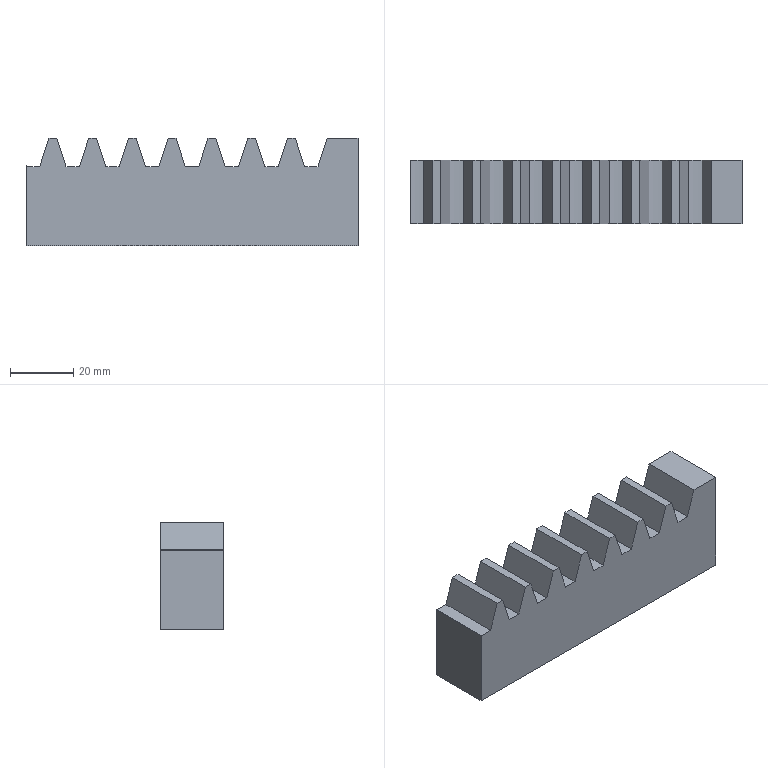Part | SolidWorks | features BaseBody 1 | 1 solid | 37 faces | box 104.88 x 20 x 34 mm | volume 61301 mm3 | plane 29 | cylinder 8 | commonest cylinder face diameters 94.224 x8
STEP:
#1=CARTESIAN_POINT('',(-7.679,369.5,-110.95));
#2=VERTEX_POINT('',#1);
#3=CARTESIAN_POINT('',(-7.753,369.5,-110.721));
#4=VERTEX_POINT('',#3);
#5=CARTESIAN_POINT('',(-7.679,369.5,-110.95));
#6=DIRECTION('',(-0.3083,0.,0.9513));
#7=VECTOR('',#6,1000.);
#8=LINE('',#5,#7);
#9=EDGE_CURVE('',#2,#4,#8,.T.);
#10=ORIENTED_EDGE('',*,*,#9,.T.);
#11=CARTESIAN_POINT('',(-7.753,369.5,-136.));
#12=VERTEX_POINT('',#11);
#13=CARTESIAN_POINT('',(-7.753,369.5,-55.957));
#14=DIRECTION('',(0.,0.,-1.));
#15=VECTOR('',#14,1000.);
#16=LINE('',#13,#15);
#17=EDGE_CURVE('',#4,#12,#16,.T.);
#18=ORIENTED_EDGE('',*,*,#17,.T.);
#19=CARTESIAN_POINT('',(97.127,369.5,-136.));
#20=VERTEX_POINT('',#19);
#21=CARTESIAN_POINT('',(52.127,369.5,-136.));
#22=DIRECTION('',(1.,0.,0.));
#23=VECTOR('',#22,1000.);
#24=LINE('',#21,#23);
#25=EDGE_CURVE('',#12,#20,#24,.T.);
#26=ORIENTED_EDGE('',*,*,#25,.T.);
#27=CARTESIAN_POINT('',(97.127,369.5,-102.));
#28=VERTEX_POINT('',#27);
#29=CARTESIAN_POINT('',(97.127,369.5,-55.957));
#30=DIRECTION('',(0.,0.,1.));
#31=VECTOR('',#30,1000.);
#32=LINE('',#29,#31);
#33=EDGE_CURVE('',#20,#28,#32,.T.);
#34=ORIENTED_EDGE('',*,*,#33,.T.);
#35=CARTESIAN_POINT('',(87.393,369.5,-102.));
#36=VERTEX_POINT('',#35);
#37=CARTESIAN_POINT('',(52.127,369.5,-102.));
#38=DIRECTION('',(-1.,0.,0.));
#39=VECTOR('',#38,1000.);
#40=LINE('',#37,#39);
#41=EDGE_CURVE('',#28,#36,#40,.T.);
#42=ORIENTED_EDGE('',*,*,#41,.T.);
#43=CARTESIAN_POINT('',(84.492,369.5,-110.95));
#44=VERTEX_POINT('',#43);
#45=CARTESIAN_POINT('',(97.545,369.5,-70.676));
#46=DIRECTION('',(-0.3083,0.,-0.9513));
#47=VECTOR('',#46,1000.);
#48=LINE('',#45,#47);
#49=EDGE_CURVE('',#36,#44,#48,.T.);
#50=ORIENTED_EDGE('',*,*,#49,.T.);
#51=CARTESIAN_POINT('',(80.241,369.5,-110.95));
#52=VERTEX_POINT('',#51);
#53=CARTESIAN_POINT('',(82.367,369.5,-63.886));
#54=DIRECTION('',(0.,1.,0.));
#55=DIRECTION('',(0.,0.,1.));
#56=AXIS2_PLACEMENT_3D('',#53,#54,#55);
#57=CIRCLE('',#56,47.112);
#58=EDGE_CURVE('',#44,#52,#57,.T.);
#59=ORIENTED_EDGE('',*,*,#58,.T.);
#60=CARTESIAN_POINT('',(77.34,369.5,-102.));
#61=VERTEX_POINT('',#60);
#62=CARTESIAN_POINT('',(80.241,369.5,-110.95));
#63=DIRECTION('',(-0.3083,0.,0.9513));
#64=VECTOR('',#63,1000.);
#65=LINE('',#62,#64);
#66=EDGE_CURVE('',#52,#61,#65,.T.);
#67=ORIENTED_EDGE('',*,*,#66,.T.);
#68=CARTESIAN_POINT('',(74.833,369.5,-102.));
#69=VERTEX_POINT('',#68);
#70=CARTESIAN_POINT('',(52.127,369.5,-102.));
#71=DIRECTION('',(-1.,0.,0.));
#72=VECTOR('',#71,1000.);
#73=LINE('',#70,#72);
#74=EDGE_CURVE('',#61,#69,#73,.T.);
#75=ORIENTED_EDGE('',*,*,#74,.T.);
#76=CARTESIAN_POINT('',(71.932,369.5,-110.95));
#77=VERTEX_POINT('',#76);
#78=CARTESIAN_POINT('',(86.178,369.5,-66.992));
#79=DIRECTION('',(-0.3083,0.,-0.9513));
#80=VECTOR('',#79,1000.);
#81=LINE('',#78,#80);
#82=EDGE_CURVE('',#69,#77,#81,.T.);
#83=ORIENTED_EDGE('',*,*,#82,.T.);
#84=CARTESIAN_POINT('',(67.681,369.5,-110.95));
#85=VERTEX_POINT('',#84);
#86=CARTESIAN_POINT('',(69.807,369.5,-63.886));
#87=DIRECTION('',(0.,1.,0.));
#88=DIRECTION('',(0.,0.,1.));
#89=AXIS2_PLACEMENT_3D('',#86,#87,#88);
#90=CIRCLE('',#89,47.112);
#91=EDGE_CURVE('',#77,#85,#90,.T.);
#92=ORIENTED_EDGE('',*,*,#91,.T.);
#93=CARTESIAN_POINT('',(64.78,369.5,-102.));
#94=VERTEX_POINT('',#93);
#95=CARTESIAN_POINT('',(67.681,369.5,-110.95));
#96=DIRECTION('',(-0.3083,0.,0.9513));
#97=VECTOR('',#96,1000.);
#98=LINE('',#95,#97);
#99=EDGE_CURVE('',#85,#94,#98,.T.);
#100=ORIENTED_EDGE('',*,*,#99,.T.);
#101=CARTESIAN_POINT('',(62.273,369.5,-102.));
#102=VERTEX_POINT('',#101);
#103=CARTESIAN_POINT('',(52.127,369.5,-102.));
#104=DIRECTION('',(-1.,0.,0.));
#105=VECTOR('',#104,1000.);
#106=LINE('',#103,#105);
#107=EDGE_CURVE('',#94,#102,#106,.T.);
#108=ORIENTED_EDGE('',*,*,#107,.T.);
#109=CARTESIAN_POINT('',(59.372,369.5,-110.95));
#110=VERTEX_POINT('',#109);
#111=CARTESIAN_POINT('',(74.812,369.5,-63.309));
#112=DIRECTION('',(-0.3083,0.,-0.9513));
#113=VECTOR('',#112,1000.);
#114=LINE('',#111,#113);
#115=EDGE_CURVE('',#102,#110,#114,.T.);
#116=ORIENTED_EDGE('',*,*,#115,.T.);
#117=CARTESIAN_POINT('',(55.121,369.5,-110.95));
#118=VERTEX_POINT('',#117);
#119=CARTESIAN_POINT('',(57.247,369.5,-63.886));
#120=DIRECTION('',(0.,1.,0.));
#121=DIRECTION('',(0.,0.,1.));
#122=AXIS2_PLACEMENT_3D('',#119,#120,#121);
#123=CIRCLE('',#122,47.112);
#124=EDGE_CURVE('',#110,#118,#123,.T.);
#125=ORIENTED_EDGE('',*,*,#124,.T.);
#126=CARTESIAN_POINT('',(52.22,369.5,-102.));
#127=VERTEX_POINT('',#126);
#128=CARTESIAN_POINT('',(55.121,369.5,-110.95));
#129=DIRECTION('',(-0.3083,0.,0.9513));
#130=VECTOR('',#129,1000.);
#131=LINE('',#128,#130);
#132=EDGE_CURVE('',#118,#127,#131,.T.);
#133=ORIENTED_EDGE('',*,*,#132,.T.);
#134=CARTESIAN_POINT('',(49.713,369.5,-102.));
#135=VERTEX_POINT('',#134);
#136=CARTESIAN_POINT('',(52.127,369.5,-102.));
#137=DIRECTION('',(-1.,0.,0.));
#138=VECTOR('',#137,1000.);
#139=LINE('',#136,#138);
#140=EDGE_CURVE('',#127,#135,#139,.T.);
#141=ORIENTED_EDGE('',*,*,#140,.T.);
#142=CARTESIAN_POINT('',(46.812,369.5,-110.95));
#143=VERTEX_POINT('',#142);
#144=CARTESIAN_POINT('',(63.446,369.5,-59.625));
#145=DIRECTION('',(-0.3083,0.,-0.9513));
#146=VECTOR('',#145,1000.);
#147=LINE('',#144,#146);
#148=EDGE_CURVE('',#135,#143,#147,.T.);
#149=ORIENTED_EDGE('',*,*,#148,.T.);
#150=CARTESIAN_POINT('',(42.561,369.5,-110.95));
#151=VERTEX_POINT('',#150);
#152=CARTESIAN_POINT('',(44.687,369.5,-63.886));
#153=DIRECTION('',(0.,1.,0.));
#154=DIRECTION('',(0.,0.,1.));
#155=AXIS2_PLACEMENT_3D('',#152,#153,#154);
#156=CIRCLE('',#155,47.112);
#157=EDGE_CURVE('',#143,#151,#156,.T.);
#158=ORIENTED_EDGE('',*,*,#157,.T.);
#159=CARTESIAN_POINT('',(39.66,369.5,-102.));
#160=VERTEX_POINT('',#159);
#161=CARTESIAN_POINT('',(42.561,369.5,-110.95));
#162=DIRECTION('',(-0.3083,0.,0.9513));
#163=VECTOR('',#162,1000.);
#164=LINE('',#161,#163);
#165=EDGE_CURVE('',#151,#160,#164,.T.);
#166=ORIENTED_EDGE('',*,*,#165,.T.);
#167=CARTESIAN_POINT('',(37.153,369.5,-102.));
#168=VERTEX_POINT('',#167);
#169=CARTESIAN_POINT('',(52.127,369.5,-102.));
#170=DIRECTION('',(-1.,0.,0.));
#171=VECTOR('',#170,1000.);
#172=LINE('',#169,#171);
#173=EDGE_CURVE('',#160,#168,#172,.T.);
#174=ORIENTED_EDGE('',*,*,#173,.T.);
#175=CARTESIAN_POINT('',(34.252,369.5,-110.95));
#176=VERTEX_POINT('',#175);
#177=CARTESIAN_POINT('',(52.08,369.5,-55.941));
#178=DIRECTION('',(-0.3083,0.,-0.9513));
#179=VECTOR('',#178,1000.);
#180=LINE('',#177,#179);
#181=EDGE_CURVE('',#168,#176,#180,.T.);
#182=ORIENTED_EDGE('',*,*,#181,.T.);
#183=CARTESIAN_POINT('',(30.001,369.5,-110.95));
#184=VERTEX_POINT('',#183);
#185=CARTESIAN_POINT('',(32.127,369.5,-63.886));
#186=DIRECTION('',(0.,1.,0.));
#187=DIRECTION('',(0.,0.,1.));
#188=AXIS2_PLACEMENT_3D('',#185,#186,#187);
#189=CIRCLE('',#188,47.112);
#190=EDGE_CURVE('',#176,#184,#189,.T.);
#191=ORIENTED_EDGE('',*,*,#190,.T.);
#192=CARTESIAN_POINT('',(27.1,369.5,-102.));
#193=VERTEX_POINT('',#192);
#194=CARTESIAN_POINT('',(30.001,369.5,-110.95));
#195=DIRECTION('',(-0.3083,0.,0.9513));
#196=VECTOR('',#195,1000.);
#197=LINE('',#194,#196);
#198=EDGE_CURVE('',#184,#193,#197,.T.);
#199=ORIENTED_EDGE('',*,*,#198,.T.);
#200=CARTESIAN_POINT('',(24.593,369.5,-102.));
#201=VERTEX_POINT('',#200);
#202=CARTESIAN_POINT('',(52.127,369.5,-102.));
#203=DIRECTION('',(-1.,0.,0.));
#204=VECTOR('',#203,1000.);
#205=LINE('',#202,#204);
#206=EDGE_CURVE('',#193,#201,#205,.T.);
#207=ORIENTED_EDGE('',*,*,#206,.T.);
#208=CARTESIAN_POINT('',(21.692,369.5,-110.95));
#209=VERTEX_POINT('',#208);
#210=CARTESIAN_POINT('',(40.714,369.5,-52.258));
#211=DIRECTION('',(-0.3083,0.,-0.9513));
#212=VECTOR('',#211,1000.);
#213=LINE('',#210,#212);
#214=EDGE_CURVE('',#201,#209,#213,.T.);
#215=ORIENTED_EDGE('',*,*,#214,.T.);
#216=CARTESIAN_POINT('',(17.441,369.5,-110.95));
#217=VERTEX_POINT('',#216);
#218=CARTESIAN_POINT('',(19.567,369.5,-63.886));
#219=DIRECTION('',(0.,1.,0.));
#220=DIRECTION('',(0.,0.,1.));
#221=AXIS2_PLACEMENT_3D('',#218,#219,#220);
#222=CIRCLE('',#221,47.112);
#223=EDGE_CURVE('',#209,#217,#222,.T.);
#224=ORIENTED_EDGE('',*,*,#223,.T.);
#225=CARTESIAN_POINT('',(14.54,369.5,-102.));
#226=VERTEX_POINT('',#225);
#227=CARTESIAN_POINT('',(17.441,369.5,-110.95));
#228=DIRECTION('',(-0.3083,0.,0.9513));
#229=VECTOR('',#228,1000.);
#230=LINE('',#227,#229);
#231=EDGE_CURVE('',#217,#226,#230,.T.);
#232=ORIENTED_EDGE('',*,*,#231,.T.);
#233=CARTESIAN_POINT('',(12.033,369.5,-102.));
#234=VERTEX_POINT('',#233);
#235=CARTESIAN_POINT('',(52.127,369.5,-102.));
#236=DIRECTION('',(-1.,0.,0.));
#237=VECTOR('',#236,1000.);
#238=LINE('',#235,#237);
#239=EDGE_CURVE('',#226,#234,#238,.T.);
#240=ORIENTED_EDGE('',*,*,#239,.T.);
#241=CARTESIAN_POINT('',(9.132,369.5,-110.95));
#242=VERTEX_POINT('',#241);
#243=CARTESIAN_POINT('',(29.347,369.5,-48.574));
#244=DIRECTION('',(-0.3083,0.,-0.9513));
#245=VECTOR('',#244,1000.);
#246=LINE('',#243,#245);
#247=EDGE_CURVE('',#234,#242,#246,.T.);
#248=ORIENTED_EDGE('',*,*,#247,.T.);
#249=CARTESIAN_POINT('',(4.881,369.5,-110.95));
#250=VERTEX_POINT('',#249);
#251=CARTESIAN_POINT('',(7.007,369.5,-63.886));
#252=DIRECTION('',(0.,1.,0.));
#253=DIRECTION('',(0.,0.,1.));
#254=AXIS2_PLACEMENT_3D('',#251,#252,#253);
#255=CIRCLE('',#254,47.112);
#256=EDGE_CURVE('',#242,#250,#255,.T.);
#257=ORIENTED_EDGE('',*,*,#256,.T.);
#258=CARTESIAN_POINT('',(1.98,369.5,-102.));
#259=VERTEX_POINT('',#258);
#260=CARTESIAN_POINT('',(4.881,369.5,-110.95));
#261=DIRECTION('',(-0.3083,0.,0.9513));
#262=VECTOR('',#261,1000.);
#263=LINE('',#260,#262);
#264=EDGE_CURVE('',#250,#259,#263,.T.);
#265=ORIENTED_EDGE('',*,*,#264,.T.);
#266=CARTESIAN_POINT('',(-0.5272,369.5,-102.));
#267=VERTEX_POINT('',#266);
#268=CARTESIAN_POINT('',(52.127,369.5,-102.));
#269=DIRECTION('',(-1.,0.,0.));
#270=VECTOR('',#269,1000.);
#271=LINE('',#268,#270);
#272=EDGE_CURVE('',#259,#267,#271,.T.);
#273=ORIENTED_EDGE('',*,*,#272,.T.);
#274=CARTESIAN_POINT('',(-3.428,369.5,-110.95));
#275=VERTEX_POINT('',#274);
#276=CARTESIAN_POINT('',(17.981,369.5,-44.891));
#277=DIRECTION('',(-0.3083,0.,-0.9513));
#278=VECTOR('',#277,1000.);
#279=LINE('',#276,#278);
#280=EDGE_CURVE('',#267,#275,#279,.T.);
#281=ORIENTED_EDGE('',*,*,#280,.T.);
#282=CARTESIAN_POINT('',(-5.553,369.5,-63.886));
#283=DIRECTION('',(0.,1.,0.));
#284=DIRECTION('',(0.,0.,1.));
#285=AXIS2_PLACEMENT_3D('',#282,#283,#284);
#286=CIRCLE('',#285,47.112);
#287=EDGE_CURVE('',#275,#2,#286,.T.);
#288=ORIENTED_EDGE('',*,*,#287,.T.);
#289=EDGE_LOOP('',(#10,#18,#26,#34,#42,#50,#59,#67,#75,#83,#92,#100,#108,#116,#125,#133,#141,#149,#158,#166,#174,#182,#191,#199,#207,#215,#224,#232,#240,#248,#257,#265,#273,#281,#288));
#290=FACE_OUTER_BOUND('',#289,.T.);
#291=CARTESIAN_POINT('',(52.127,369.5,-55.957));
#292=DIRECTION('',(0.,-1.,0.));
#293=DIRECTION('',(0.,0.,-1.));
#294=AXIS2_PLACEMENT_3D('',#291,#292,#293);
#295=PLANE('',#294);
#296=ADVANCED_FACE('',(#290),#295,.T.);
#297=CARTESIAN_POINT('',(-7.753,389.5,-110.721));
#298=VERTEX_POINT('',#297);
#299=CARTESIAN_POINT('',(-7.753,379.5,-110.721));
#300=DIRECTION('',(0.,-1.,0.));
#301=VECTOR('',#300,1000.);
#302=LINE('',#299,#301);
#303=EDGE_CURVE('',#298,#4,#302,.T.);
#304=ORIENTED_EDGE('',*,*,#303,.F.);
#305=CARTESIAN_POINT('',(-7.753,389.5,-136.));
#306=VERTEX_POINT('',#305);
#307=CARTESIAN_POINT('',(-7.753,389.5,-178.522));
#308=DIRECTION('',(0.,0.,1.));
#309=VECTOR('',#308,1000.);
#310=LINE('',#307,#309);
#311=EDGE_CURVE('',#306,#298,#310,.T.);
#312=ORIENTED_EDGE('',*,*,#311,.F.);
#313=CARTESIAN_POINT('',(-7.753,379.5,-136.));
#314=DIRECTION('',(0.,1.,0.));
#315=VECTOR('',#314,1000.);
#316=LINE('',#313,#315);
#317=EDGE_CURVE('',#12,#306,#316,.T.);
#318=ORIENTED_EDGE('',*,*,#317,.F.);
#319=ORIENTED_EDGE('',*,*,#17,.F.);
#320=EDGE_LOOP('',(#304,#312,#318,#319));
#321=FACE_OUTER_BOUND('',#320,.T.);
#322=CARTESIAN_POINT('',(-7.753,379.5,-178.522));
#323=DIRECTION('',(1.,0.,0.));
#324=DIRECTION('',(0.,0.,-1.));
#325=AXIS2_PLACEMENT_3D('',#322,#323,#324);
#326=PLANE('',#325);
#327=ADVANCED_FACE('',(#321),#326,.F.);
#328=CARTESIAN_POINT('',(-7.679,389.5,-110.95));
#329=VERTEX_POINT('',#328);
#330=CARTESIAN_POINT('',(-7.894,389.5,-110.286));
#331=DIRECTION('',(-0.3083,0.,0.9513));
#332=VECTOR('',#331,1000.);
#333=LINE('',#330,#332);
#334=EDGE_CURVE('',#329,#298,#333,.T.);
#335=ORIENTED_EDGE('',*,*,#334,.T.);
#336=ORIENTED_EDGE('',*,*,#303,.T.);
#337=ORIENTED_EDGE('',*,*,#9,.F.);
#338=CARTESIAN_POINT('',(-7.679,294.5,-110.95));
#339=DIRECTION('',(0.,1.,0.));
#340=VECTOR('',#339,1000.);
#341=LINE('',#338,#340);
#342=EDGE_CURVE('',#2,#329,#341,.T.);
#343=ORIENTED_EDGE('',*,*,#342,.T.);
#344=EDGE_LOOP('',(#335,#336,#337,#343));
#345=FACE_OUTER_BOUND('',#344,.T.);
#346=CARTESIAN_POINT('',(-7.894,294.5,-110.286));
#347=DIRECTION('',(0.9513,0.,0.3083));
#348=DIRECTION('',(0.3083,0.,-0.9513));
#349=AXIS2_PLACEMENT_3D('',#346,#347,#348);
#350=PLANE('',#349);
#351=ADVANCED_FACE('',(#345),#350,.T.);
#352=ORIENTED_EDGE('',*,*,#287,.F.);
#353=CARTESIAN_POINT('',(-3.428,389.5,-110.95));
#354=VERTEX_POINT('',#353);
#355=CARTESIAN_POINT('',(-3.428,379.5,-110.95));
#356=DIRECTION('',(0.,-1.,0.));
#357=VECTOR('',#356,1000.);
#358=LINE('',#355,#357);
#359=EDGE_CURVE('',#354,#275,#358,.T.);
#360=ORIENTED_EDGE('',*,*,#359,.F.);
#361=CARTESIAN_POINT('',(-5.553,389.5,-63.886));
#362=DIRECTION('',(0.,-1.,0.));
#363=DIRECTION('',(0.,0.,1.));
#364=AXIS2_PLACEMENT_3D('',#361,#362,#363);
#365=CIRCLE('',#364,47.112);
#366=EDGE_CURVE('',#329,#354,#365,.T.);
#367=ORIENTED_EDGE('',*,*,#366,.F.);
#368=ORIENTED_EDGE('',*,*,#342,.F.);
#369=EDGE_LOOP('',(#352,#360,#367,#368));
#370=FACE_OUTER_BOUND('',#369,.T.);
#371=CARTESIAN_POINT('',(-5.553,379.5,-63.886));
#372=DIRECTION('',(0.,1.,0.));
#373=DIRECTION('',(0.,0.,1.));
#374=AXIS2_PLACEMENT_3D('',#371,#372,#373);
#375=CYLINDRICAL_SURFACE('',#374,47.112);
#376=ADVANCED_FACE('',(#370),#375,.F.);
#377=CARTESIAN_POINT('',(-0.5272,389.5,-102.));
#378=VERTEX_POINT('',#377);
#379=CARTESIAN_POINT('',(-0.5272,294.5,-102.));
#380=DIRECTION('',(0.,1.,0.));
#381=VECTOR('',#380,1000.);
#382=LINE('',#379,#381);
#383=EDGE_CURVE('',#267,#378,#382,.T.);
#384=ORIENTED_EDGE('',*,*,#383,.T.);
#385=CARTESIAN_POINT('',(-1.094,389.5,-103.748));
#386=DIRECTION('',(-0.3083,0.,-0.9513));
#387=VECTOR('',#386,1000.);
#388=LINE('',#385,#387);
#389=EDGE_CURVE('',#378,#354,#388,.T.);
#390=ORIENTED_EDGE('',*,*,#389,.T.);
#391=ORIENTED_EDGE('',*,*,#359,.T.);
#392=ORIENTED_EDGE('',*,*,#280,.F.);
#393=EDGE_LOOP('',(#384,#390,#391,#392));
#394=FACE_OUTER_BOUND('',#393,.T.);
#395=CARTESIAN_POINT('',(-1.094,294.5,-103.748));
#396=DIRECTION('',(-0.9513,0.,0.3083));
#397=DIRECTION('',(0.3083,0.,0.9513));
#398=AXIS2_PLACEMENT_3D('',#395,#396,#397);
#399=PLANE('',#398);
#400=ADVANCED_FACE('',(#394),#399,.T.);
#401=ORIENTED_EDGE('',*,*,#272,.F.);
#402=CARTESIAN_POINT('',(1.98,389.5,-102.));
#403=VERTEX_POINT('',#402);
#404=CARTESIAN_POINT('',(1.98,389.115,-102.));
#405=DIRECTION('',(0.,-1.,0.));
#406=VECTOR('',#405,1000.);
#407=LINE('',#404,#406);
#408=EDGE_CURVE('',#403,#259,#407,.T.);
#409=ORIENTED_EDGE('',*,*,#408,.F.);
#410=CARTESIAN_POINT('',(106.357,389.5,-102.));
#411=DIRECTION('',(1.,0.,0.));
#412=VECTOR('',#411,1000.);
#413=LINE('',#410,#412);
#414=EDGE_CURVE('',#378,#403,#413,.T.);
#415=ORIENTED_EDGE('',*,*,#414,.F.);
#416=ORIENTED_EDGE('',*,*,#383,.F.);
#417=EDGE_LOOP('',(#401,#409,#415,#416));
#418=FACE_OUTER_BOUND('',#417,.T.);
#419=CARTESIAN_POINT('',(106.357,389.115,-102.));
#420=DIRECTION('',(0.,0.,-1.));
#421=DIRECTION('',(-1.,0.,0.));
#422=AXIS2_PLACEMENT_3D('',#419,#420,#421);
#423=PLANE('',#422);
#424=ADVANCED_FACE('',(#418),#423,.F.);
#425=CARTESIAN_POINT('',(4.881,389.5,-110.95));
#426=VERTEX_POINT('',#425);
#427=CARTESIAN_POINT('',(4.881,369.5,-110.95));
#428=DIRECTION('',(0.,1.,0.));
#429=VECTOR('',#428,1000.);
#430=LINE('',#427,#429);
#431=EDGE_CURVE('',#250,#426,#430,.T.);
#432=ORIENTED_EDGE('',*,*,#431,.T.);
#433=CARTESIAN_POINT('',(4.666,389.5,-110.286));
#434=DIRECTION('',(-0.3083,0.,0.9513));
#435=VECTOR('',#434,1000.);
#436=LINE('',#433,#435);
#437=EDGE_CURVE('',#426,#403,#436,.T.);
#438=ORIENTED_EDGE('',*,*,#437,.T.);
#439=ORIENTED_EDGE('',*,*,#408,.T.);
#440=ORIENTED_EDGE('',*,*,#264,.F.);
#441=EDGE_LOOP('',(#432,#438,#439,#440));
#442=FACE_OUTER_BOUND('',#441,.T.);
#443=CARTESIAN_POINT('',(4.666,294.5,-110.286));
#444=DIRECTION('',(0.9513,0.,0.3083));
#445=DIRECTION('',(0.3083,0.,-0.9513));
#446=AXIS2_PLACEMENT_3D('',#443,#444,#445);
#447=PLANE('',#446);
#448=ADVANCED_FACE('',(#442),#447,.T.);
#449=ORIENTED_EDGE('',*,*,#256,.F.);
#450=CARTESIAN_POINT('',(9.132,389.5,-110.95));
#451=VERTEX_POINT('',#450);
#452=CARTESIAN_POINT('',(9.132,379.5,-110.95));
#453=DIRECTION('',(0.,-1.,0.));
#454=VECTOR('',#453,1000.);
#455=LINE('',#452,#454);
#456=EDGE_CURVE('',#451,#242,#455,.T.);
#457=ORIENTED_EDGE('',*,*,#456,.F.);
#458=CARTESIAN_POINT('',(7.007,389.5,-63.886));
#459=DIRECTION('',(0.,-1.,0.));
#460=DIRECTION('',(0.,0.,1.));
#461=AXIS2_PLACEMENT_3D('',#458,#459,#460);
#462=CIRCLE('',#461,47.112);
#463=EDGE_CURVE('',#426,#451,#462,.T.);
#464=ORIENTED_EDGE('',*,*,#463,.F.);
#465=ORIENTED_EDGE('',*,*,#431,.F.);
#466=EDGE_LOOP('',(#449,#457,#464,#465));
#467=FACE_OUTER_BOUND('',#466,.T.);
#468=CARTESIAN_POINT('',(7.007,379.5,-63.886));
#469=DIRECTION('',(0.,1.,0.));
#470=DIRECTION('',(0.,0.,1.));
#471=AXIS2_PLACEMENT_3D('',#468,#469,#470);
#472=CYLINDRICAL_SURFACE('',#471,47.112);
#473=ADVANCED_FACE('',(#467),#472,.F.);
#474=CARTESIAN_POINT('',(12.033,389.5,-102.));
#475=VERTEX_POINT('',#474);
#476=CARTESIAN_POINT('',(12.033,294.5,-102.));
#477=DIRECTION('',(0.,1.,0.));
#478=VECTOR('',#477,1000.);
#479=LINE('',#476,#478);
#480=EDGE_CURVE('',#234,#475,#479,.T.);
#481=ORIENTED_EDGE('',*,*,#480,.T.);
#482=CARTESIAN_POINT('',(11.466,389.5,-103.748));
#483=DIRECTION('',(-0.3083,0.,-0.9513));
#484=VECTOR('',#483,1000.);
#485=LINE('',#482,#484);
#486=EDGE_CURVE('',#475,#451,#485,.T.);
#487=ORIENTED_EDGE('',*,*,#486,.T.);
#488=ORIENTED_EDGE('',*,*,#456,.T.);
#489=ORIENTED_EDGE('',*,*,#247,.F.);
#490=EDGE_LOOP('',(#481,#487,#488,#489));
#491=FACE_OUTER_BOUND('',#490,.T.);
#492=CARTESIAN_POINT('',(11.466,294.5,-103.748));
#493=DIRECTION('',(-0.9513,0.,0.3083));
#494=DIRECTION('',(0.3083,0.,0.9513));
#495=AXIS2_PLACEMENT_3D('',#492,#493,#494);
#496=PLANE('',#495);
#497=ADVANCED_FACE('',(#491),#496,.T.);
#498=ORIENTED_EDGE('',*,*,#239,.F.);
#499=CARTESIAN_POINT('',(14.54,389.5,-102.));
#500=VERTEX_POINT('',#499);
#501=CARTESIAN_POINT('',(14.54,389.115,-102.));
#502=DIRECTION('',(0.,-1.,0.));
#503=VECTOR('',#502,1000.);
#504=LINE('',#501,#503);
#505=EDGE_CURVE('',#500,#226,#504,.T.);
#506=ORIENTED_EDGE('',*,*,#505,.F.);
#507=CARTESIAN_POINT('',(106.357,389.5,-102.));
#508=DIRECTION('',(1.,0.,0.));
#509=VECTOR('',#508,1000.);
#510=LINE('',#507,#509);
#511=EDGE_CURVE('',#475,#500,#510,.T.);
#512=ORIENTED_EDGE('',*,*,#511,.F.);
#513=ORIENTED_EDGE('',*,*,#480,.F.);
#514=EDGE_LOOP('',(#498,#506,#512,#513));
#515=FACE_OUTER_BOUND('',#514,.T.);
#516=CARTESIAN_POINT('',(106.357,389.115,-102.));
#517=DIRECTION('',(0.,0.,-1.));
#518=DIRECTION('',(-1.,0.,0.));
#519=AXIS2_PLACEMENT_3D('',#516,#517,#518);
#520=PLANE('',#519);
#521=ADVANCED_FACE('',(#515),#520,.F.);
#522=CARTESIAN_POINT('',(17.441,389.5,-110.95));
#523=VERTEX_POINT('',#522);
#524=CARTESIAN_POINT('',(17.441,369.5,-110.95));
#525=DIRECTION('',(0.,1.,0.));
#526=VECTOR('',#525,1000.);
#527=LINE('',#524,#526);
#528=EDGE_CURVE('',#217,#523,#527,.T.);
#529=ORIENTED_EDGE('',*,*,#528,.T.);
#530=CARTESIAN_POINT('',(17.226,389.5,-110.286));
#531=DIRECTION('',(-0.3083,0.,0.9513));
#532=VECTOR('',#531,1000.);
#533=LINE('',#530,#532);
#534=EDGE_CURVE('',#523,#500,#533,.T.);
#535=ORIENTED_EDGE('',*,*,#534,.T.);
#536=ORIENTED_EDGE('',*,*,#505,.T.);
#537=ORIENTED_EDGE('',*,*,#231,.F.);
#538=EDGE_LOOP('',(#529,#535,#536,#537));
#539=FACE_OUTER_BOUND('',#538,.T.);
#540=CARTESIAN_POINT('',(17.226,294.5,-110.286));
#541=DIRECTION('',(0.9513,0.,0.3083));
#542=DIRECTION('',(0.3083,0.,-0.9513));
#543=AXIS2_PLACEMENT_3D('',#540,#541,#542);
#544=PLANE('',#543);
#545=ADVANCED_FACE('',(#539),#544,.T.);
#546=ORIENTED_EDGE('',*,*,#223,.F.);
#547=CARTESIAN_POINT('',(21.692,389.5,-110.95));
#548=VERTEX_POINT('',#547);
#549=CARTESIAN_POINT('',(21.692,379.5,-110.95));
#550=DIRECTION('',(0.,-1.,0.));
#551=VECTOR('',#550,1000.);
#552=LINE('',#549,#551);
#553=EDGE_CURVE('',#548,#209,#552,.T.);
#554=ORIENTED_EDGE('',*,*,#553,.F.);
#555=CARTESIAN_POINT('',(19.567,389.5,-63.886));
#556=DIRECTION('',(0.,-1.,0.));
#557=DIRECTION('',(0.,0.,1.));
#558=AXIS2_PLACEMENT_3D('',#555,#556,#557);
#559=CIRCLE('',#558,47.112);
#560=EDGE_CURVE('',#523,#548,#559,.T.);
#561=ORIENTED_EDGE('',*,*,#560,.F.);
#562=ORIENTED_EDGE('',*,*,#528,.F.);
#563=EDGE_LOOP('',(#546,#554,#561,#562));
#564=FACE_OUTER_BOUND('',#563,.T.);
#565=CARTESIAN_POINT('',(19.567,379.5,-63.886));
#566=DIRECTION('',(0.,1.,0.));
#567=DIRECTION('',(0.,0.,1.));
#568=AXIS2_PLACEMENT_3D('',#565,#566,#567);
#569=CYLINDRICAL_SURFACE('',#568,47.112);
#570=ADVANCED_FACE('',(#564),#569,.F.);
#571=CARTESIAN_POINT('',(24.593,389.5,-102.));
#572=VERTEX_POINT('',#571);
#573=CARTESIAN_POINT('',(24.593,294.5,-102.));
#574=DIRECTION('',(0.,1.,0.));
#575=VECTOR('',#574,1000.);
#576=LINE('',#573,#575);
#577=EDGE_CURVE('',#201,#572,#576,.T.);
#578=ORIENTED_EDGE('',*,*,#577,.T.);
#579=CARTESIAN_POINT('',(24.026,389.5,-103.748));
#580=DIRECTION('',(-0.3083,0.,-0.9513));
#581=VECTOR('',#580,1000.);
#582=LINE('',#579,#581);
#583=EDGE_CURVE('',#572,#548,#582,.T.);
#584=ORIENTED_EDGE('',*,*,#583,.T.);
#585=ORIENTED_EDGE('',*,*,#553,.T.);
#586=ORIENTED_EDGE('',*,*,#214,.F.);
#587=EDGE_LOOP('',(#578,#584,#585,#586));
#588=FACE_OUTER_BOUND('',#587,.T.);
#589=CARTESIAN_POINT('',(24.026,294.5,-103.748));
#590=DIRECTION('',(-0.9513,0.,0.3083));
#591=DIRECTION('',(0.3083,0.,0.9513));
#592=AXIS2_PLACEMENT_3D('',#589,#590,#591);
#593=PLANE('',#592);
#594=ADVANCED_FACE('',(#588),#593,.T.);
#595=ORIENTED_EDGE('',*,*,#206,.F.);
#596=CARTESIAN_POINT('',(27.1,389.5,-102.));
#597=VERTEX_POINT('',#596);
#598=CARTESIAN_POINT('',(27.1,389.115,-102.));
#599=DIRECTION('',(0.,-1.,0.));
#600=VECTOR('',#599,1000.);
#601=LINE('',#598,#600);
#602=EDGE_CURVE('',#597,#193,#601,.T.);
#603=ORIENTED_EDGE('',*,*,#602,.F.);
#604=CARTESIAN_POINT('',(106.357,389.5,-102.));
#605=DIRECTION('',(1.,0.,0.));
#606=VECTOR('',#605,1000.);
#607=LINE('',#604,#606);
#608=EDGE_CURVE('',#572,#597,#607,.T.);
#609=ORIENTED_EDGE('',*,*,#608,.F.);
#610=ORIENTED_EDGE('',*,*,#577,.F.);
#611=EDGE_LOOP('',(#595,#603,#609,#610));
#612=FACE_OUTER_BOUND('',#611,.T.);
#613=CARTESIAN_POINT('',(106.357,389.115,-102.));
#614=DIRECTION('',(0.,0.,-1.));
#615=DIRECTION('',(-1.,0.,0.));
#616=AXIS2_PLACEMENT_3D('',#613,#614,#615);
#617=PLANE('',#616);
#618=ADVANCED_FACE('',(#612),#617,.F.);
#619=CARTESIAN_POINT('',(30.001,389.5,-110.95));
#620=VERTEX_POINT('',#619);
#621=CARTESIAN_POINT('',(30.001,369.5,-110.95));
#622=DIRECTION('',(0.,1.,0.));
#623=VECTOR('',#622,1000.);
#624=LINE('',#621,#623);
#625=EDGE_CURVE('',#184,#620,#624,.T.);
#626=ORIENTED_EDGE('',*,*,#625,.T.);
#627=CARTESIAN_POINT('',(29.786,389.5,-110.286));
#628=DIRECTION('',(-0.3083,0.,0.9513));
#629=VECTOR('',#628,1000.);
#630=LINE('',#627,#629);
#631=EDGE_CURVE('',#620,#597,#630,.T.);
#632=ORIENTED_EDGE('',*,*,#631,.T.);
#633=ORIENTED_EDGE('',*,*,#602,.T.);
#634=ORIENTED_EDGE('',*,*,#198,.F.);
#635=EDGE_LOOP('',(#626,#632,#633,#634));
#636=FACE_OUTER_BOUND('',#635,.T.);
#637=CARTESIAN_POINT('',(29.786,294.5,-110.286));
#638=DIRECTION('',(0.9513,0.,0.3083));
#639=DIRECTION('',(0.3083,0.,-0.9513));
#640=AXIS2_PLACEMENT_3D('',#637,#638,#639);
#641=PLANE('',#640);
#642=ADVANCED_FACE('',(#636),#641,.T.);
#643=ORIENTED_EDGE('',*,*,#190,.F.);
#644=CARTESIAN_POINT('',(34.252,389.5,-110.95));
#645=VERTEX_POINT('',#644);
#646=CARTESIAN_POINT('',(34.252,379.5,-110.95));
#647=DIRECTION('',(0.,-1.,0.));
#648=VECTOR('',#647,1000.);
#649=LINE('',#646,#648);
#650=EDGE_CURVE('',#645,#176,#649,.T.);
#651=ORIENTED_EDGE('',*,*,#650,.F.);
#652=CARTESIAN_POINT('',(32.127,389.5,-63.886));
#653=DIRECTION('',(0.,-1.,0.));
#654=DIRECTION('',(0.,0.,1.));
#655=AXIS2_PLACEMENT_3D('',#652,#653,#654);
#656=CIRCLE('',#655,47.112);
#657=EDGE_CURVE('',#620,#645,#656,.T.);
#658=ORIENTED_EDGE('',*,*,#657,.F.);
#659=ORIENTED_EDGE('',*,*,#625,.F.);
#660=EDGE_LOOP('',(#643,#651,#658,#659));
#661=FACE_OUTER_BOUND('',#660,.T.);
#662=CARTESIAN_POINT('',(32.127,379.5,-63.886));
#663=DIRECTION('',(0.,1.,0.));
#664=DIRECTION('',(0.,0.,1.));
#665=AXIS2_PLACEMENT_3D('',#662,#663,#664);
#666=CYLINDRICAL_SURFACE('',#665,47.112);
#667=ADVANCED_FACE('',(#661),#666,.F.);
#668=CARTESIAN_POINT('',(37.153,389.5,-102.));
#669=VERTEX_POINT('',#668);
#670=CARTESIAN_POINT('',(37.153,294.5,-102.));
#671=DIRECTION('',(0.,1.,0.));
#672=VECTOR('',#671,1000.);
#673=LINE('',#670,#672);
#674=EDGE_CURVE('',#168,#669,#673,.T.);
#675=ORIENTED_EDGE('',*,*,#674,.T.);
#676=CARTESIAN_POINT('',(36.586,389.5,-103.748));
#677=DIRECTION('',(-0.3083,0.,-0.9513));
#678=VECTOR('',#677,1000.);
#679=LINE('',#676,#678);
#680=EDGE_CURVE('',#669,#645,#679,.T.);
#681=ORIENTED_EDGE('',*,*,#680,.T.);
#682=ORIENTED_EDGE('',*,*,#650,.T.);
#683=ORIENTED_EDGE('',*,*,#181,.F.);
#684=EDGE_LOOP('',(#675,#681,#682,#683));
#685=FACE_OUTER_BOUND('',#684,.T.);
#686=CARTESIAN_POINT('',(36.586,294.5,-103.748));
#687=DIRECTION('',(-0.9513,0.,0.3083));
#688=DIRECTION('',(0.3083,0.,0.9513));
#689=AXIS2_PLACEMENT_3D('',#686,#687,#688);
#690=PLANE('',#689);
#691=ADVANCED_FACE('',(#685),#690,.T.);
#692=ORIENTED_EDGE('',*,*,#173,.F.);
#693=CARTESIAN_POINT('',(39.66,389.5,-102.));
#694=VERTEX_POINT('',#693);
#695=CARTESIAN_POINT('',(39.66,389.115,-102.));
#696=DIRECTION('',(0.,-1.,0.));
#697=VECTOR('',#696,1000.);
#698=LINE('',#695,#697);
#699=EDGE_CURVE('',#694,#160,#698,.T.);
#700=ORIENTED_EDGE('',*,*,#699,.F.);
#701=CARTESIAN_POINT('',(106.357,389.5,-102.));
#702=DIRECTION('',(1.,0.,0.));
#703=VECTOR('',#702,1000.);
#704=LINE('',#701,#703);
#705=EDGE_CURVE('',#669,#694,#704,.T.);
#706=ORIENTED_EDGE('',*,*,#705,.F.);
#707=ORIENTED_EDGE('',*,*,#674,.F.);
#708=EDGE_LOOP('',(#692,#700,#706,#707));
#709=FACE_OUTER_BOUND('',#708,.T.);
#710=CARTESIAN_POINT('',(106.357,389.115,-102.));
#711=DIRECTION('',(0.,0.,-1.));
#712=DIRECTION('',(-1.,0.,0.));
#713=AXIS2_PLACEMENT_3D('',#710,#711,#712);
#714=PLANE('',#713);
#715=ADVANCED_FACE('',(#709),#714,.F.);
#716=CARTESIAN_POINT('',(42.561,389.5,-110.95));
#717=VERTEX_POINT('',#716);
#718=CARTESIAN_POINT('',(42.561,369.5,-110.95));
#719=DIRECTION('',(0.,1.,0.));
#720=VECTOR('',#719,1000.);
#721=LINE('',#718,#720);
#722=EDGE_CURVE('',#151,#717,#721,.T.);
#723=ORIENTED_EDGE('',*,*,#722,.T.);
#724=CARTESIAN_POINT('',(42.346,389.5,-110.286));
#725=DIRECTION('',(-0.3083,0.,0.9513));
#726=VECTOR('',#725,1000.);
#727=LINE('',#724,#726);
#728=EDGE_CURVE('',#717,#694,#727,.T.);
#729=ORIENTED_EDGE('',*,*,#728,.T.);
#730=ORIENTED_EDGE('',*,*,#699,.T.);
#731=ORIENTED_EDGE('',*,*,#165,.F.);
#732=EDGE_LOOP('',(#723,#729,#730,#731));
#733=FACE_OUTER_BOUND('',#732,.T.);
#734=CARTESIAN_POINT('',(42.346,294.5,-110.286));
#735=DIRECTION('',(0.9513,0.,0.3083));
#736=DIRECTION('',(0.3083,0.,-0.9513));
#737=AXIS2_PLACEMENT_3D('',#734,#735,#736);
#738=PLANE('',#737);
#739=ADVANCED_FACE('',(#733),#738,.T.);
#740=ORIENTED_EDGE('',*,*,#157,.F.);
#741=CARTESIAN_POINT('',(46.812,389.5,-110.95));
#742=VERTEX_POINT('',#741);
#743=CARTESIAN_POINT('',(46.812,379.5,-110.95));
#744=DIRECTION('',(0.,-1.,0.));
#745=VECTOR('',#744,1000.);
#746=LINE('',#743,#745);
#747=EDGE_CURVE('',#742,#143,#746,.T.);
#748=ORIENTED_EDGE('',*,*,#747,.F.);
#749=CARTESIAN_POINT('',(44.687,389.5,-63.886));
#750=DIRECTION('',(0.,-1.,0.));
#751=DIRECTION('',(0.,0.,1.));
#752=AXIS2_PLACEMENT_3D('',#749,#750,#751);
#753=CIRCLE('',#752,47.112);
#754=EDGE_CURVE('',#717,#742,#753,.T.);
#755=ORIENTED_EDGE('',*,*,#754,.F.);
#756=ORIENTED_EDGE('',*,*,#722,.F.);
#757=EDGE_LOOP('',(#740,#748,#755,#756));
#758=FACE_OUTER_BOUND('',#757,.T.);
#759=CARTESIAN_POINT('',(44.687,379.5,-63.886));
#760=DIRECTION('',(0.,1.,0.));
#761=DIRECTION('',(0.,0.,1.));
#762=AXIS2_PLACEMENT_3D('',#759,#760,#761);
#763=CYLINDRICAL_SURFACE('',#762,47.112);
#764=ADVANCED_FACE('',(#758),#763,.F.);
#765=CARTESIAN_POINT('',(49.713,389.5,-102.));
#766=VERTEX_POINT('',#765);
#767=CARTESIAN_POINT('',(49.713,294.5,-102.));
#768=DIRECTION('',(0.,1.,0.));
#769=VECTOR('',#768,1000.);
#770=LINE('',#767,#769);
#771=EDGE_CURVE('',#135,#766,#770,.T.);
#772=ORIENTED_EDGE('',*,*,#771,.T.);
#773=CARTESIAN_POINT('',(49.146,389.5,-103.748));
#774=DIRECTION('',(-0.3083,0.,-0.9513));
#775=VECTOR('',#774,1000.);
#776=LINE('',#773,#775);
#777=EDGE_CURVE('',#766,#742,#776,.T.);
#778=ORIENTED_EDGE('',*,*,#777,.T.);
#779=ORIENTED_EDGE('',*,*,#747,.T.);
#780=ORIENTED_EDGE('',*,*,#148,.F.);
#781=EDGE_LOOP('',(#772,#778,#779,#780));
#782=FACE_OUTER_BOUND('',#781,.T.);
#783=CARTESIAN_POINT('',(49.146,294.5,-103.748));
#784=DIRECTION('',(-0.9513,0.,0.3083));
#785=DIRECTION('',(0.3083,0.,0.9513));
#786=AXIS2_PLACEMENT_3D('',#783,#784,#785);
#787=PLANE('',#786);
#788=ADVANCED_FACE('',(#782),#787,.T.);
#789=ORIENTED_EDGE('',*,*,#140,.F.);
#790=CARTESIAN_POINT('',(52.22,389.5,-102.));
#791=VERTEX_POINT('',#790);
#792=CARTESIAN_POINT('',(52.22,389.115,-102.));
#793=DIRECTION('',(0.,-1.,0.));
#794=VECTOR('',#793,1000.);
#795=LINE('',#792,#794);
#796=EDGE_CURVE('',#791,#127,#795,.T.);
#797=ORIENTED_EDGE('',*,*,#796,.F.);
#798=CARTESIAN_POINT('',(106.357,389.5,-102.));
#799=DIRECTION('',(1.,0.,0.));
#800=VECTOR('',#799,1000.);
#801=LINE('',#798,#800);
#802=EDGE_CURVE('',#766,#791,#801,.T.);
#803=ORIENTED_EDGE('',*,*,#802,.F.);
#804=ORIENTED_EDGE('',*,*,#771,.F.);
#805=EDGE_LOOP('',(#789,#797,#803,#804));
#806=FACE_OUTER_BOUND('',#805,.T.);
#807=CARTESIAN_POINT('',(106.357,389.115,-102.));
#808=DIRECTION('',(0.,0.,-1.));
#809=DIRECTION('',(-1.,0.,0.));
#810=AXIS2_PLACEMENT_3D('',#807,#808,#809);
#811=PLANE('',#810);
#812=ADVANCED_FACE('',(#806),#811,.F.);
#813=CARTESIAN_POINT('',(55.121,389.5,-110.95));
#814=VERTEX_POINT('',#813);
#815=CARTESIAN_POINT('',(55.121,369.5,-110.95));
#816=DIRECTION('',(0.,1.,0.));
#817=VECTOR('',#816,1000.);
#818=LINE('',#815,#817);
#819=EDGE_CURVE('',#118,#814,#818,.T.);
#820=ORIENTED_EDGE('',*,*,#819,.T.);
#821=CARTESIAN_POINT('',(54.906,389.5,-110.286));
#822=DIRECTION('',(-0.3083,0.,0.9513));
#823=VECTOR('',#822,1000.);
#824=LINE('',#821,#823);
#825=EDGE_CURVE('',#814,#791,#824,.T.);
#826=ORIENTED_EDGE('',*,*,#825,.T.);
#827=ORIENTED_EDGE('',*,*,#796,.T.);
#828=ORIENTED_EDGE('',*,*,#132,.F.);
#829=EDGE_LOOP('',(#820,#826,#827,#828));
#830=FACE_OUTER_BOUND('',#829,.T.);
#831=CARTESIAN_POINT('',(54.906,294.5,-110.286));
#832=DIRECTION('',(0.9513,0.,0.3083));
#833=DIRECTION('',(0.3083,0.,-0.9513));
#834=AXIS2_PLACEMENT_3D('',#831,#832,#833);
#835=PLANE('',#834);
#836=ADVANCED_FACE('',(#830),#835,.T.);
#837=ORIENTED_EDGE('',*,*,#124,.F.);
#838=CARTESIAN_POINT('',(59.372,389.5,-110.95));
#839=VERTEX_POINT('',#838);
#840=CARTESIAN_POINT('',(59.372,379.5,-110.95));
#841=DIRECTION('',(0.,-1.,0.));
#842=VECTOR('',#841,1000.);
#843=LINE('',#840,#842);
#844=EDGE_CURVE('',#839,#110,#843,.T.);
#845=ORIENTED_EDGE('',*,*,#844,.F.);
#846=CARTESIAN_POINT('',(57.247,389.5,-63.886));
#847=DIRECTION('',(0.,-1.,0.));
#848=DIRECTION('',(0.,0.,1.));
#849=AXIS2_PLACEMENT_3D('',#846,#847,#848);
#850=CIRCLE('',#849,47.112);
#851=EDGE_CURVE('',#814,#839,#850,.T.);
#852=ORIENTED_EDGE('',*,*,#851,.F.);
#853=ORIENTED_EDGE('',*,*,#819,.F.);
#854=EDGE_LOOP('',(#837,#845,#852,#853));
#855=FACE_OUTER_BOUND('',#854,.T.);
#856=CARTESIAN_POINT('',(57.247,379.5,-63.886));
#857=DIRECTION('',(0.,1.,0.));
#858=DIRECTION('',(0.,0.,1.));
#859=AXIS2_PLACEMENT_3D('',#856,#857,#858);
#860=CYLINDRICAL_SURFACE('',#859,47.112);
#861=ADVANCED_FACE('',(#855),#860,.F.);
#862=CARTESIAN_POINT('',(62.273,389.5,-102.));
#863=VERTEX_POINT('',#862);
#864=CARTESIAN_POINT('',(62.273,294.5,-102.));
#865=DIRECTION('',(0.,1.,0.));
#866=VECTOR('',#865,1000.);
#867=LINE('',#864,#866);
#868=EDGE_CURVE('',#102,#863,#867,.T.);
#869=ORIENTED_EDGE('',*,*,#868,.T.);
#870=CARTESIAN_POINT('',(61.706,389.5,-103.748));
#871=DIRECTION('',(-0.3083,0.,-0.9513));
#872=VECTOR('',#871,1000.);
#873=LINE('',#870,#872);
#874=EDGE_CURVE('',#863,#839,#873,.T.);
#875=ORIENTED_EDGE('',*,*,#874,.T.);
#876=ORIENTED_EDGE('',*,*,#844,.T.);
#877=ORIENTED_EDGE('',*,*,#115,.F.);
#878=EDGE_LOOP('',(#869,#875,#876,#877));
#879=FACE_OUTER_BOUND('',#878,.T.);
#880=CARTESIAN_POINT('',(61.706,294.5,-103.748));
#881=DIRECTION('',(-0.9513,0.,0.3083));
#882=DIRECTION('',(0.3083,0.,0.9513));
#883=AXIS2_PLACEMENT_3D('',#880,#881,#882);
#884=PLANE('',#883);
#885=ADVANCED_FACE('',(#879),#884,.T.);
#886=ORIENTED_EDGE('',*,*,#107,.F.);
#887=CARTESIAN_POINT('',(64.78,389.5,-102.));
#888=VERTEX_POINT('',#887);
#889=CARTESIAN_POINT('',(64.78,389.115,-102.));
#890=DIRECTION('',(0.,-1.,0.));
#891=VECTOR('',#890,1000.);
#892=LINE('',#889,#891);
#893=EDGE_CURVE('',#888,#94,#892,.T.);
#894=ORIENTED_EDGE('',*,*,#893,.F.);
#895=CARTESIAN_POINT('',(106.357,389.5,-102.));
#896=DIRECTION('',(1.,0.,0.));
#897=VECTOR('',#896,1000.);
#898=LINE('',#895,#897);
#899=EDGE_CURVE('',#863,#888,#898,.T.);
#900=ORIENTED_EDGE('',*,*,#899,.F.);
#901=ORIENTED_EDGE('',*,*,#868,.F.);
#902=EDGE_LOOP('',(#886,#894,#900,#901));
#903=FACE_OUTER_BOUND('',#902,.T.);
#904=CARTESIAN_POINT('',(106.357,389.115,-102.));
#905=DIRECTION('',(0.,0.,-1.));
#906=DIRECTION('',(-1.,0.,0.));
#907=AXIS2_PLACEMENT_3D('',#904,#905,#906);
#908=PLANE('',#907);
#909=ADVANCED_FACE('',(#903),#908,.F.);
#910=CARTESIAN_POINT('',(67.681,389.5,-110.95));
#911=VERTEX_POINT('',#910);
#912=CARTESIAN_POINT('',(67.681,369.5,-110.95));
#913=DIRECTION('',(0.,1.,0.));
#914=VECTOR('',#913,1000.);
#915=LINE('',#912,#914);
#916=EDGE_CURVE('',#85,#911,#915,.T.);
#917=ORIENTED_EDGE('',*,*,#916,.T.);
#918=CARTESIAN_POINT('',(67.466,389.5,-110.286));
#919=DIRECTION('',(-0.3083,0.,0.9513));
#920=VECTOR('',#919,1000.);
#921=LINE('',#918,#920);
#922=EDGE_CURVE('',#911,#888,#921,.T.);
#923=ORIENTED_EDGE('',*,*,#922,.T.);
#924=ORIENTED_EDGE('',*,*,#893,.T.);
#925=ORIENTED_EDGE('',*,*,#99,.F.);
#926=EDGE_LOOP('',(#917,#923,#924,#925));
#927=FACE_OUTER_BOUND('',#926,.T.);
#928=CARTESIAN_POINT('',(67.466,294.5,-110.286));
#929=DIRECTION('',(0.9513,0.,0.3083));
#930=DIRECTION('',(0.3083,0.,-0.9513));
#931=AXIS2_PLACEMENT_3D('',#928,#929,#930);
#932=PLANE('',#931);
#933=ADVANCED_FACE('',(#927),#932,.T.);
#934=ORIENTED_EDGE('',*,*,#91,.F.);
#935=CARTESIAN_POINT('',(71.932,389.5,-110.95));
#936=VERTEX_POINT('',#935);
#937=CARTESIAN_POINT('',(71.932,379.5,-110.95));
#938=DIRECTION('',(0.,-1.,0.));
#939=VECTOR('',#938,1000.);
#940=LINE('',#937,#939);
#941=EDGE_CURVE('',#936,#77,#940,.T.);
#942=ORIENTED_EDGE('',*,*,#941,.F.);
#943=CARTESIAN_POINT('',(69.807,389.5,-63.886));
#944=DIRECTION('',(0.,-1.,0.));
#945=DIRECTION('',(0.,0.,1.));
#946=AXIS2_PLACEMENT_3D('',#943,#944,#945);
#947=CIRCLE('',#946,47.112);
#948=EDGE_CURVE('',#911,#936,#947,.T.);
#949=ORIENTED_EDGE('',*,*,#948,.F.);
#950=ORIENTED_EDGE('',*,*,#916,.F.);
#951=EDGE_LOOP('',(#934,#942,#949,#950));
#952=FACE_OUTER_BOUND('',#951,.T.);
#953=CARTESIAN_POINT('',(69.807,379.5,-63.886));
#954=DIRECTION('',(0.,1.,0.));
#955=DIRECTION('',(0.,0.,1.));
#956=AXIS2_PLACEMENT_3D('',#953,#954,#955);
#957=CYLINDRICAL_SURFACE('',#956,47.112);
#958=ADVANCED_FACE('',(#952),#957,.F.);
#959=CARTESIAN_POINT('',(74.833,389.5,-102.));
#960=VERTEX_POINT('',#959);
#961=CARTESIAN_POINT('',(74.833,294.5,-102.));
#962=DIRECTION('',(0.,1.,0.));
#963=VECTOR('',#962,1000.);
#964=LINE('',#961,#963);
#965=EDGE_CURVE('',#69,#960,#964,.T.);
#966=ORIENTED_EDGE('',*,*,#965,.T.);
#967=CARTESIAN_POINT('',(74.266,389.5,-103.748));
#968=DIRECTION('',(-0.3083,0.,-0.9513));
#969=VECTOR('',#968,1000.);
#970=LINE('',#967,#969);
#971=EDGE_CURVE('',#960,#936,#970,.T.);
#972=ORIENTED_EDGE('',*,*,#971,.T.);
#973=ORIENTED_EDGE('',*,*,#941,.T.);
#974=ORIENTED_EDGE('',*,*,#82,.F.);
#975=EDGE_LOOP('',(#966,#972,#973,#974));
#976=FACE_OUTER_BOUND('',#975,.T.);
#977=CARTESIAN_POINT('',(74.266,294.5,-103.748));
#978=DIRECTION('',(-0.9513,0.,0.3083));
#979=DIRECTION('',(0.3083,0.,0.9513));
#980=AXIS2_PLACEMENT_3D('',#977,#978,#979);
#981=PLANE('',#980);
#982=ADVANCED_FACE('',(#976),#981,.T.);
#983=ORIENTED_EDGE('',*,*,#74,.F.);
#984=CARTESIAN_POINT('',(77.34,389.5,-102.));
#985=VERTEX_POINT('',#984);
#986=CARTESIAN_POINT('',(77.34,389.115,-102.));
#987=DIRECTION('',(0.,-1.,0.));
#988=VECTOR('',#987,1000.);
#989=LINE('',#986,#988);
#990=EDGE_CURVE('',#985,#61,#989,.T.);
#991=ORIENTED_EDGE('',*,*,#990,.F.);
#992=CARTESIAN_POINT('',(106.357,389.5,-102.));
#993=DIRECTION('',(1.,0.,0.));
#994=VECTOR('',#993,1000.);
#995=LINE('',#992,#994);
#996=EDGE_CURVE('',#960,#985,#995,.T.);
#997=ORIENTED_EDGE('',*,*,#996,.F.);
#998=ORIENTED_EDGE('',*,*,#965,.F.);
#999=EDGE_LOOP('',(#983,#991,#997,#998));
#1000=FACE_OUTER_BOUND('',#999,.T.);
#1001=CARTESIAN_POINT('',(106.357,389.115,-102.));
#1002=DIRECTION('',(0.,0.,-1.));
#1003=DIRECTION('',(-1.,0.,0.));
#1004=AXIS2_PLACEMENT_3D('',#1001,#1002,#1003);
#1005=PLANE('',#1004);
#1006=ADVANCED_FACE('',(#1000),#1005,.F.);
#1007=CARTESIAN_POINT('',(80.241,389.5,-110.95));
#1008=VERTEX_POINT('',#1007);
#1009=CARTESIAN_POINT('',(80.241,369.5,-110.95));
#1010=DIRECTION('',(0.,1.,0.));
#1011=VECTOR('',#1010,1000.);
#1012=LINE('',#1009,#1011);
#1013=EDGE_CURVE('',#52,#1008,#1012,.T.);
#1014=ORIENTED_EDGE('',*,*,#1013,.T.);
#1015=CARTESIAN_POINT('',(80.026,389.5,-110.286));
#1016=DIRECTION('',(-0.3083,0.,0.9513));
#1017=VECTOR('',#1016,1000.);
#1018=LINE('',#1015,#1017);
#1019=EDGE_CURVE('',#1008,#985,#1018,.T.);
#1020=ORIENTED_EDGE('',*,*,#1019,.T.);
#1021=ORIENTED_EDGE('',*,*,#990,.T.);
#1022=ORIENTED_EDGE('',*,*,#66,.F.);
#1023=EDGE_LOOP('',(#1014,#1020,#1021,#1022));
#1024=FACE_OUTER_BOUND('',#1023,.T.);
#1025=CARTESIAN_POINT('',(80.026,294.5,-110.286));
#1026=DIRECTION('',(0.9513,0.,0.3083));
#1027=DIRECTION('',(0.3083,0.,-0.9513));
#1028=AXIS2_PLACEMENT_3D('',#1025,#1026,#1027);
#1029=PLANE('',#1028);
#1030=ADVANCED_FACE('',(#1024),#1029,.T.);
#1031=ORIENTED_EDGE('',*,*,#58,.F.);
#1032=CARTESIAN_POINT('',(84.492,389.5,-110.95));
#1033=VERTEX_POINT('',#1032);
#1034=CARTESIAN_POINT('',(84.492,379.5,-110.95));
#1035=DIRECTION('',(0.,-1.,0.));
#1036=VECTOR('',#1035,1000.);
#1037=LINE('',#1034,#1036);
#1038=EDGE_CURVE('',#1033,#44,#1037,.T.);
#1039=ORIENTED_EDGE('',*,*,#1038,.F.);
#1040=CARTESIAN_POINT('',(82.367,389.5,-63.886));
#1041=DIRECTION('',(0.,-1.,0.));
#1042=DIRECTION('',(0.,0.,1.));
#1043=AXIS2_PLACEMENT_3D('',#1040,#1041,#1042);
#1044=CIRCLE('',#1043,47.112);
#1045=EDGE_CURVE('',#1008,#1033,#1044,.T.);
#1046=ORIENTED_EDGE('',*,*,#1045,.F.);
#1047=ORIENTED_EDGE('',*,*,#1013,.F.);
#1048=EDGE_LOOP('',(#1031,#1039,#1046,#1047));
#1049=FACE_OUTER_BOUND('',#1048,.T.);
#1050=CARTESIAN_POINT('',(82.367,379.5,-63.886));
#1051=DIRECTION('',(0.,1.,0.));
#1052=DIRECTION('',(0.,0.,1.));
#1053=AXIS2_PLACEMENT_3D('',#1050,#1051,#1052);
#1054=CYLINDRICAL_SURFACE('',#1053,47.112);
#1055=ADVANCED_FACE('',(#1049),#1054,.F.);
#1056=CARTESIAN_POINT('',(87.393,389.5,-102.));
#1057=VERTEX_POINT('',#1056);
#1058=CARTESIAN_POINT('',(87.393,294.5,-102.));
#1059=DIRECTION('',(0.,1.,0.));
#1060=VECTOR('',#1059,1000.);
#1061=LINE('',#1058,#1060);
#1062=EDGE_CURVE('',#36,#1057,#1061,.T.);
#1063=ORIENTED_EDGE('',*,*,#1062,.T.);
#1064=CARTESIAN_POINT('',(86.826,389.5,-103.748));
#1065=DIRECTION('',(-0.3083,0.,-0.9513));
#1066=VECTOR('',#1065,1000.);
#1067=LINE('',#1064,#1066);
#1068=EDGE_CURVE('',#1057,#1033,#1067,.T.);
#1069=ORIENTED_EDGE('',*,*,#1068,.T.);
#1070=ORIENTED_EDGE('',*,*,#1038,.T.);
#1071=ORIENTED_EDGE('',*,*,#49,.F.);
#1072=EDGE_LOOP('',(#1063,#1069,#1070,#1071));
#1073=FACE_OUTER_BOUND('',#1072,.T.);
#1074=CARTESIAN_POINT('',(86.826,294.5,-103.748));
#1075=DIRECTION('',(-0.9513,0.,0.3083));
#1076=DIRECTION('',(0.3083,0.,0.9513));
#1077=AXIS2_PLACEMENT_3D('',#1074,#1075,#1076);
#1078=PLANE('',#1077);
#1079=ADVANCED_FACE('',(#1073),#1078,.T.);
#1080=ORIENTED_EDGE('',*,*,#41,.F.);
#1081=CARTESIAN_POINT('',(97.127,389.5,-102.));
#1082=VERTEX_POINT('',#1081);
#1083=CARTESIAN_POINT('',(97.127,389.115,-102.));
#1084=DIRECTION('',(0.,-1.,0.));
#1085=VECTOR('',#1084,1000.);
#1086=LINE('',#1083,#1085);
#1087=EDGE_CURVE('',#1082,#28,#1086,.T.);
#1088=ORIENTED_EDGE('',*,*,#1087,.F.);
#1089=CARTESIAN_POINT('',(106.357,389.5,-102.));
#1090=DIRECTION('',(1.,0.,0.));
#1091=VECTOR('',#1090,1000.);
#1092=LINE('',#1089,#1091);
#1093=EDGE_CURVE('',#1057,#1082,#1092,.T.);
#1094=ORIENTED_EDGE('',*,*,#1093,.F.);
#1095=ORIENTED_EDGE('',*,*,#1062,.F.);
#1096=EDGE_LOOP('',(#1080,#1088,#1094,#1095));
#1097=FACE_OUTER_BOUND('',#1096,.T.);
#1098=CARTESIAN_POINT('',(106.357,389.115,-102.));
#1099=DIRECTION('',(0.,0.,-1.));
#1100=DIRECTION('',(-1.,0.,0.));
#1101=AXIS2_PLACEMENT_3D('',#1098,#1099,#1100);
#1102=PLANE('',#1101);
#1103=ADVANCED_FACE('',(#1097),#1102,.F.);
#1104=ORIENTED_EDGE('',*,*,#33,.F.);
#1105=CARTESIAN_POINT('',(97.127,389.5,-136.));
#1106=VERTEX_POINT('',#1105);
#1107=CARTESIAN_POINT('',(97.127,379.5,-136.));
#1108=DIRECTION('',(0.,-1.,0.));
#1109=VECTOR('',#1108,1000.);
#1110=LINE('',#1107,#1109);
#1111=EDGE_CURVE('',#1106,#20,#1110,.T.);
#1112=ORIENTED_EDGE('',*,*,#1111,.F.);
#1113=CARTESIAN_POINT('',(97.127,389.5,-6.478));
#1114=DIRECTION('',(0.,0.,-1.));
#1115=VECTOR('',#1114,1000.);
#1116=LINE('',#1113,#1115);
#1117=EDGE_CURVE('',#1082,#1106,#1116,.T.);
#1118=ORIENTED_EDGE('',*,*,#1117,.F.);
#1119=ORIENTED_EDGE('',*,*,#1087,.T.);
#1120=EDGE_LOOP('',(#1104,#1112,#1118,#1119));
#1121=FACE_OUTER_BOUND('',#1120,.T.);
#1122=CARTESIAN_POINT('',(97.127,379.5,-6.478));
#1123=DIRECTION('',(-1.,0.,0.));
#1124=DIRECTION('',(0.,0.,1.));
#1125=AXIS2_PLACEMENT_3D('',#1122,#1123,#1124);
#1126=PLANE('',#1125);
#1127=ADVANCED_FACE('',(#1121),#1126,.F.);
#1128=ORIENTED_EDGE('',*,*,#25,.F.);
#1129=ORIENTED_EDGE('',*,*,#317,.T.);
#1130=CARTESIAN_POINT('',(106.357,389.5,-136.));
#1131=DIRECTION('',(1.,0.,0.));
#1132=VECTOR('',#1131,1000.);
#1133=LINE('',#1130,#1132);
#1134=EDGE_CURVE('',#306,#1106,#1133,.T.);
#1135=ORIENTED_EDGE('',*,*,#1134,.T.);
#1136=ORIENTED_EDGE('',*,*,#1111,.T.);
#1137=EDGE_LOOP('',(#1128,#1129,#1135,#1136));
#1138=FACE_OUTER_BOUND('',#1137,.T.);
#1139=CARTESIAN_POINT('',(106.357,389.115,-136.));
#1140=DIRECTION('',(0.,0.,-1.));
#1141=DIRECTION('',(-1.,0.,0.));
#1142=AXIS2_PLACEMENT_3D('',#1139,#1140,#1141);
#1143=PLANE('',#1142);
#1144=ADVANCED_FACE('',(#1138),#1143,.T.);
#1145=ORIENTED_EDGE('',*,*,#1134,.F.);
#1146=ORIENTED_EDGE('',*,*,#311,.T.);
#1147=ORIENTED_EDGE('',*,*,#334,.F.);
#1148=ORIENTED_EDGE('',*,*,#366,.T.);
#1149=ORIENTED_EDGE('',*,*,#389,.F.);
#1150=ORIENTED_EDGE('',*,*,#414,.T.);
#1151=ORIENTED_EDGE('',*,*,#437,.F.);
#1152=ORIENTED_EDGE('',*,*,#463,.T.);
#1153=ORIENTED_EDGE('',*,*,#486,.F.);
#1154=ORIENTED_EDGE('',*,*,#511,.T.);
#1155=ORIENTED_EDGE('',*,*,#534,.F.);
#1156=ORIENTED_EDGE('',*,*,#560,.T.);
#1157=ORIENTED_EDGE('',*,*,#583,.F.);
#1158=ORIENTED_EDGE('',*,*,#608,.T.);
#1159=ORIENTED_EDGE('',*,*,#631,.F.);
#1160=ORIENTED_EDGE('',*,*,#657,.T.);
#1161=ORIENTED_EDGE('',*,*,#680,.F.);
#1162=ORIENTED_EDGE('',*,*,#705,.T.);
#1163=ORIENTED_EDGE('',*,*,#728,.F.);
#1164=ORIENTED_EDGE('',*,*,#754,.T.);
#1165=ORIENTED_EDGE('',*,*,#777,.F.);
#1166=ORIENTED_EDGE('',*,*,#802,.T.);
#1167=ORIENTED_EDGE('',*,*,#825,.F.);
#1168=ORIENTED_EDGE('',*,*,#851,.T.);
#1169=ORIENTED_EDGE('',*,*,#874,.F.);
#1170=ORIENTED_EDGE('',*,*,#899,.T.);
#1171=ORIENTED_EDGE('',*,*,#922,.F.);
#1172=ORIENTED_EDGE('',*,*,#948,.T.);
#1173=ORIENTED_EDGE('',*,*,#971,.F.);
#1174=ORIENTED_EDGE('',*,*,#996,.T.);
#1175=ORIENTED_EDGE('',*,*,#1019,.F.);
#1176=ORIENTED_EDGE('',*,*,#1045,.T.);
#1177=ORIENTED_EDGE('',*,*,#1068,.F.);
#1178=ORIENTED_EDGE('',*,*,#1093,.T.);
#1179=ORIENTED_EDGE('',*,*,#1117,.T.);
#1180=EDGE_LOOP('',(#1145,#1146,#1147,#1148,#1149,#1150,#1151,#1152,#1153,#1154,#1155,#1156,#1157,#1158,#1159,#1160,#1161,#1162,#1163,#1164,#1165,#1166,#1167,#1168,#1169,#1170,#1171,#1172,#1173,#1174,#1175,#1176,#1177,#1178,#1179));
#1181=FACE_OUTER_BOUND('',#1180,.T.);
#1182=CARTESIAN_POINT('',(26.511,389.5,212.615));
#1183=DIRECTION('',(0.,1.,0.));
#1184=DIRECTION('',(0.,0.,1.));
#1185=AXIS2_PLACEMENT_3D('',#1182,#1183,#1184);
#1186=PLANE('',#1185);
#1187=ADVANCED_FACE('',(#1181),#1186,.T.);
#1188=CLOSED_SHELL('',(#296,#327,#351,#376,#400,#424,#448,#473,#497,#521,#545,#570,#594,#618,#642,#667,#691,#715,#739,#764,#788,#812,#836,#861,#885,#909,#933,#958,#982,#1006,#1030,#1055,#1079,#1103,#1127,#1144,#1187));
#1189=MANIFOLD_SOLID_BREP('',#1188);
#1190=CARTESIAN_POINT('',(0.,0.,0.));
#1191=DIRECTION('',(0.,0.,1.));
#1192=DIRECTION('',(1.,0.,0.));
#1193=AXIS2_PLACEMENT_3D('',#1190,#1191,#1192);
#1194=(LENGTH_UNIT()NAMED_UNIT(*)SI_UNIT(.MILLI.,.METRE.));
#1195=UNCERTAINTY_MEASURE_WITH_UNIT(LENGTH_MEASURE(0.00001),#1194,'','');
#1196=(NAMED_UNIT(*)PLANE_ANGLE_UNIT()SI_UNIT($,.RADIAN.));
#1197=(NAMED_UNIT(*)SI_UNIT($,.STERADIAN.)SOLID_ANGLE_UNIT());
#1198=(GEOMETRIC_REPRESENTATION_CONTEXT(3)GLOBAL_UNCERTAINTY_ASSIGNED_CONTEXT((#1195))GLOBAL_UNIT_ASSIGNED_CONTEXT((#1194,#1196,#1197))REPRESENTATION_CONTEXT('',''));
#1199=ADVANCED_BREP_SHAPE_REPRESENTATION('',(#1189,#1193),#1198);